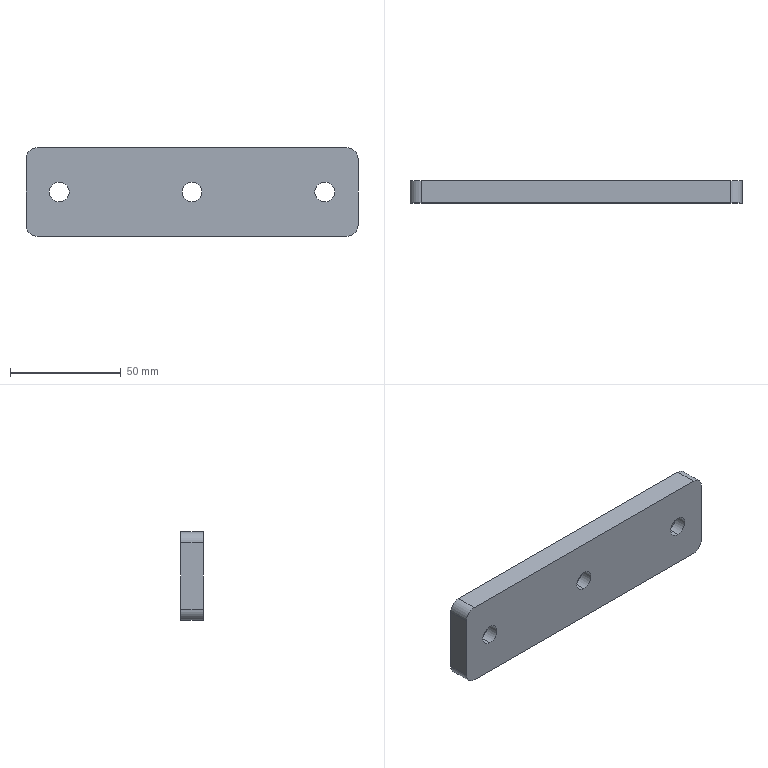Part | SolidWorks | features LPattern 2, Extrusion 1, Fillet 1, HoleWzd 1, ICE 1 | 1 solid | 22 faces | box 150 x 10 x 40 mm | volume 56843 mm3 | cylinder 10 | cone 6 | plane 6 | commonest cylinder face diameters 9 x6 10 x4
STEP:
#1=CARTESIAN_POINT('',(75.,5.7,-24.5));
#2=VERTEX_POINT('',#1);
#3=CARTESIAN_POINT('',(75.,5.7,-15.5));
#4=VERTEX_POINT('',#3);
#5=CARTESIAN_POINT('',(75.,5.7,-20.));
#6=DIRECTION('',(0.,1.,0.));
#7=DIRECTION('',(0.,0.,1.));
#8=AXIS2_PLACEMENT_3D('',#5,#6,#7);
#9=CIRCLE('',#8,4.5);
#10=EDGE_CURVE('',#2,#4,#9,.T.);
#11=ORIENTED_EDGE('',*,*,#10,.F.);
#12=CARTESIAN_POINT('',(75.,10.,-28.8));
#13=VERTEX_POINT('',#12);
#14=CARTESIAN_POINT('',(75.,10.,-28.8));
#15=DIRECTION('',(0.,0.7071,-0.7071));
#16=VECTOR('',#15,1000.);
#17=LINE('',#14,#16);
#18=EDGE_CURVE('',#2,#13,#17,.T.);
#19=ORIENTED_EDGE('',*,*,#18,.T.);
#20=CARTESIAN_POINT('',(75.,10.,-11.2));
#21=VERTEX_POINT('',#20);
#22=CARTESIAN_POINT('',(75.,10.,-20.));
#23=DIRECTION('',(0.,1.,0.));
#24=DIRECTION('',(0.,0.,1.));
#25=AXIS2_PLACEMENT_3D('',#22,#23,#24);
#26=CIRCLE('',#25,8.8);
#27=EDGE_CURVE('',#13,#21,#26,.T.);
#28=ORIENTED_EDGE('',*,*,#27,.T.);
#29=CARTESIAN_POINT('',(75.,10.,-11.2));
#30=DIRECTION('',(0.,0.7071,0.7071));
#31=VECTOR('',#30,1000.);
#32=LINE('',#29,#31);
#33=EDGE_CURVE('',#4,#21,#32,.T.);
#34=ORIENTED_EDGE('',*,*,#33,.F.);
#35=EDGE_LOOP('',(#11,#19,#28,#34));
#36=FACE_OUTER_BOUND('',#35,.T.);
#37=CARTESIAN_POINT('',(75.,10.,-20.));
#38=DIRECTION('',(0.,1.,0.));
#39=DIRECTION('',(0.,0.,1.));
#40=AXIS2_PLACEMENT_3D('',#37,#38,#39);
#41=CONICAL_SURFACE('',#40,8.8,0.7854);
#42=ADVANCED_FACE('',(#36),#41,.F.);
#43=CARTESIAN_POINT('',(75.,0.,-15.5));
#44=VERTEX_POINT('',#43);
#45=CARTESIAN_POINT('',(75.,0.,-24.5));
#46=VERTEX_POINT('',#45);
#47=CARTESIAN_POINT('',(75.,0.,-20.));
#48=DIRECTION('',(0.,-1.,0.));
#49=DIRECTION('',(0.,0.,-1.));
#50=AXIS2_PLACEMENT_3D('',#47,#48,#49);
#51=CIRCLE('',#50,4.5);
#52=EDGE_CURVE('',#44,#46,#51,.T.);
#53=ORIENTED_EDGE('',*,*,#52,.T.);
#54=CARTESIAN_POINT('',(75.,10.,-24.5));
#55=DIRECTION('',(0.,1.,0.));
#56=VECTOR('',#55,1000.);
#57=LINE('',#54,#56);
#58=EDGE_CURVE('',#46,#2,#57,.T.);
#59=ORIENTED_EDGE('',*,*,#58,.T.);
#60=ORIENTED_EDGE('',*,*,#10,.T.);
#61=CARTESIAN_POINT('',(75.,10.,-15.5));
#62=DIRECTION('',(0.,1.,0.));
#63=VECTOR('',#62,1000.);
#64=LINE('',#61,#63);
#65=EDGE_CURVE('',#44,#4,#64,.T.);
#66=ORIENTED_EDGE('',*,*,#65,.F.);
#67=EDGE_LOOP('',(#53,#59,#60,#66));
#68=FACE_OUTER_BOUND('',#67,.T.);
#69=CARTESIAN_POINT('',(75.,10.,-20.));
#70=DIRECTION('',(0.,1.,0.));
#71=DIRECTION('',(0.,0.,1.));
#72=AXIS2_PLACEMENT_3D('',#69,#70,#71);
#73=CYLINDRICAL_SURFACE('',#72,4.5);
#74=ADVANCED_FACE('',(#68),#73,.F.);
#75=CARTESIAN_POINT('',(15.,5.7,-24.5));
#76=VERTEX_POINT('',#75);
#77=CARTESIAN_POINT('',(15.,5.7,-15.5));
#78=VERTEX_POINT('',#77);
#79=CARTESIAN_POINT('',(15.,5.7,-20.));
#80=DIRECTION('',(0.,1.,0.));
#81=DIRECTION('',(0.,0.,1.));
#82=AXIS2_PLACEMENT_3D('',#79,#80,#81);
#83=CIRCLE('',#82,4.5);
#84=EDGE_CURVE('',#76,#78,#83,.T.);
#85=ORIENTED_EDGE('',*,*,#84,.F.);
#86=CARTESIAN_POINT('',(15.,10.,-28.8));
#87=VERTEX_POINT('',#86);
#88=CARTESIAN_POINT('',(15.,10.,-28.8));
#89=DIRECTION('',(0.,0.7071,-0.7071));
#90=VECTOR('',#89,1000.);
#91=LINE('',#88,#90);
#92=EDGE_CURVE('',#76,#87,#91,.T.);
#93=ORIENTED_EDGE('',*,*,#92,.T.);
#94=CARTESIAN_POINT('',(15.,10.,-11.2));
#95=VERTEX_POINT('',#94);
#96=CARTESIAN_POINT('',(15.,10.,-20.));
#97=DIRECTION('',(0.,1.,0.));
#98=DIRECTION('',(0.,0.,1.));
#99=AXIS2_PLACEMENT_3D('',#96,#97,#98);
#100=CIRCLE('',#99,8.8);
#101=EDGE_CURVE('',#87,#95,#100,.T.);
#102=ORIENTED_EDGE('',*,*,#101,.T.);
#103=CARTESIAN_POINT('',(15.,10.,-11.2));
#104=DIRECTION('',(0.,0.7071,0.7071));
#105=VECTOR('',#104,1000.);
#106=LINE('',#103,#105);
#107=EDGE_CURVE('',#78,#95,#106,.T.);
#108=ORIENTED_EDGE('',*,*,#107,.F.);
#109=EDGE_LOOP('',(#85,#93,#102,#108));
#110=FACE_OUTER_BOUND('',#109,.T.);
#111=CARTESIAN_POINT('',(15.,10.,-20.));
#112=DIRECTION('',(0.,1.,0.));
#113=DIRECTION('',(0.,0.,1.));
#114=AXIS2_PLACEMENT_3D('',#111,#112,#113);
#115=CONICAL_SURFACE('',#114,8.8,0.7854);
#116=ADVANCED_FACE('',(#110),#115,.F.);
#117=CARTESIAN_POINT('',(15.,0.,-15.5));
#118=VERTEX_POINT('',#117);
#119=CARTESIAN_POINT('',(15.,0.,-24.5));
#120=VERTEX_POINT('',#119);
#121=CARTESIAN_POINT('',(15.,0.,-20.));
#122=DIRECTION('',(0.,-1.,0.));
#123=DIRECTION('',(0.,0.,-1.));
#124=AXIS2_PLACEMENT_3D('',#121,#122,#123);
#125=CIRCLE('',#124,4.5);
#126=EDGE_CURVE('',#118,#120,#125,.T.);
#127=ORIENTED_EDGE('',*,*,#126,.T.);
#128=CARTESIAN_POINT('',(15.,10.,-24.5));
#129=DIRECTION('',(0.,1.,0.));
#130=VECTOR('',#129,1000.);
#131=LINE('',#128,#130);
#132=EDGE_CURVE('',#120,#76,#131,.T.);
#133=ORIENTED_EDGE('',*,*,#132,.T.);
#134=ORIENTED_EDGE('',*,*,#84,.T.);
#135=CARTESIAN_POINT('',(15.,10.,-15.5));
#136=DIRECTION('',(0.,1.,0.));
#137=VECTOR('',#136,1000.);
#138=LINE('',#135,#137);
#139=EDGE_CURVE('',#118,#78,#138,.T.);
#140=ORIENTED_EDGE('',*,*,#139,.F.);
#141=EDGE_LOOP('',(#127,#133,#134,#140));
#142=FACE_OUTER_BOUND('',#141,.T.);
#143=CARTESIAN_POINT('',(15.,10.,-20.));
#144=DIRECTION('',(0.,1.,0.));
#145=DIRECTION('',(0.,0.,1.));
#146=AXIS2_PLACEMENT_3D('',#143,#144,#145);
#147=CYLINDRICAL_SURFACE('',#146,4.5);
#148=ADVANCED_FACE('',(#142),#147,.F.);
#149=CARTESIAN_POINT('',(135.,5.7,-24.5));
#150=VERTEX_POINT('',#149);
#151=CARTESIAN_POINT('',(135.,5.7,-15.5));
#152=VERTEX_POINT('',#151);
#153=CARTESIAN_POINT('',(135.,5.7,-20.));
#154=DIRECTION('',(0.,1.,0.));
#155=DIRECTION('',(0.,0.,1.));
#156=AXIS2_PLACEMENT_3D('',#153,#154,#155);
#157=CIRCLE('',#156,4.5);
#158=EDGE_CURVE('',#150,#152,#157,.T.);
#159=ORIENTED_EDGE('',*,*,#158,.F.);
#160=CARTESIAN_POINT('',(135.,10.,-28.8));
#161=VERTEX_POINT('',#160);
#162=CARTESIAN_POINT('',(135.,10.,-28.8));
#163=DIRECTION('',(0.,0.7071,-0.7071));
#164=VECTOR('',#163,1000.);
#165=LINE('',#162,#164);
#166=EDGE_CURVE('',#150,#161,#165,.T.);
#167=ORIENTED_EDGE('',*,*,#166,.T.);
#168=CARTESIAN_POINT('',(135.,10.,-11.2));
#169=VERTEX_POINT('',#168);
#170=CARTESIAN_POINT('',(135.,10.,-20.));
#171=DIRECTION('',(0.,1.,0.));
#172=DIRECTION('',(0.,0.,1.));
#173=AXIS2_PLACEMENT_3D('',#170,#171,#172);
#174=CIRCLE('',#173,8.8);
#175=EDGE_CURVE('',#161,#169,#174,.T.);
#176=ORIENTED_EDGE('',*,*,#175,.T.);
#177=CARTESIAN_POINT('',(135.,10.,-11.2));
#178=DIRECTION('',(0.,0.7071,0.7071));
#179=VECTOR('',#178,1000.);
#180=LINE('',#177,#179);
#181=EDGE_CURVE('',#152,#169,#180,.T.);
#182=ORIENTED_EDGE('',*,*,#181,.F.);
#183=EDGE_LOOP('',(#159,#167,#176,#182));
#184=FACE_OUTER_BOUND('',#183,.T.);
#185=CARTESIAN_POINT('',(135.,10.,-20.));
#186=DIRECTION('',(0.,1.,0.));
#187=DIRECTION('',(0.,0.,1.));
#188=AXIS2_PLACEMENT_3D('',#185,#186,#187);
#189=CONICAL_SURFACE('',#188,8.8,0.7854);
#190=ADVANCED_FACE('',(#184),#189,.F.);
#191=CARTESIAN_POINT('',(135.,0.,-15.5));
#192=VERTEX_POINT('',#191);
#193=CARTESIAN_POINT('',(135.,0.,-24.5));
#194=VERTEX_POINT('',#193);
#195=CARTESIAN_POINT('',(135.,0.,-20.));
#196=DIRECTION('',(0.,-1.,0.));
#197=DIRECTION('',(0.,0.,-1.));
#198=AXIS2_PLACEMENT_3D('',#195,#196,#197);
#199=CIRCLE('',#198,4.5);
#200=EDGE_CURVE('',#192,#194,#199,.T.);
#201=ORIENTED_EDGE('',*,*,#200,.T.);
#202=CARTESIAN_POINT('',(135.,10.,-24.5));
#203=DIRECTION('',(0.,1.,0.));
#204=VECTOR('',#203,1000.);
#205=LINE('',#202,#204);
#206=EDGE_CURVE('',#194,#150,#205,.T.);
#207=ORIENTED_EDGE('',*,*,#206,.T.);
#208=ORIENTED_EDGE('',*,*,#158,.T.);
#209=CARTESIAN_POINT('',(135.,10.,-15.5));
#210=DIRECTION('',(0.,1.,0.));
#211=VECTOR('',#210,1000.);
#212=LINE('',#209,#211);
#213=EDGE_CURVE('',#192,#152,#212,.T.);
#214=ORIENTED_EDGE('',*,*,#213,.F.);
#215=EDGE_LOOP('',(#201,#207,#208,#214));
#216=FACE_OUTER_BOUND('',#215,.T.);
#217=CARTESIAN_POINT('',(135.,10.,-20.));
#218=DIRECTION('',(0.,1.,0.));
#219=DIRECTION('',(0.,0.,1.));
#220=AXIS2_PLACEMENT_3D('',#217,#218,#219);
#221=CYLINDRICAL_SURFACE('',#220,4.5);
#222=ADVANCED_FACE('',(#216),#221,.F.);
#223=CARTESIAN_POINT('',(0.,10.,-35.));
#224=VERTEX_POINT('',#223);
#225=CARTESIAN_POINT('',(0.,10.,-5.));
#226=VERTEX_POINT('',#225);
#227=CARTESIAN_POINT('',(0.,10.,0.));
#228=DIRECTION('',(0.,0.,1.));
#229=VECTOR('',#228,1000.);
#230=LINE('',#227,#229);
#231=EDGE_CURVE('',#224,#226,#230,.T.);
#232=ORIENTED_EDGE('',*,*,#231,.F.);
#233=CARTESIAN_POINT('',(0.,0.,-35.));
#234=VERTEX_POINT('',#233);
#235=CARTESIAN_POINT('',(0.,10.,-35.));
#236=DIRECTION('',(0.,-1.,0.));
#237=VECTOR('',#236,1000.);
#238=LINE('',#235,#237);
#239=EDGE_CURVE('',#224,#234,#238,.T.);
#240=ORIENTED_EDGE('',*,*,#239,.T.);
#241=CARTESIAN_POINT('',(0.,0.,-5.));
#242=VERTEX_POINT('',#241);
#243=CARTESIAN_POINT('',(0.,0.,0.));
#244=DIRECTION('',(0.,0.,1.));
#245=VECTOR('',#244,1000.);
#246=LINE('',#243,#245);
#247=EDGE_CURVE('',#234,#242,#246,.T.);
#248=ORIENTED_EDGE('',*,*,#247,.T.);
#249=CARTESIAN_POINT('',(0.,10.,-5.));
#250=DIRECTION('',(0.,1.,0.));
#251=VECTOR('',#250,1000.);
#252=LINE('',#249,#251);
#253=EDGE_CURVE('',#242,#226,#252,.T.);
#254=ORIENTED_EDGE('',*,*,#253,.T.);
#255=EDGE_LOOP('',(#232,#240,#248,#254));
#256=FACE_OUTER_BOUND('',#255,.T.);
#257=CARTESIAN_POINT('',(0.,10.,0.));
#258=DIRECTION('',(1.,0.,0.));
#259=DIRECTION('',(0.,0.,-1.));
#260=AXIS2_PLACEMENT_3D('',#257,#258,#259);
#261=PLANE('',#260);
#262=ADVANCED_FACE('',(#256),#261,.F.);
#263=CARTESIAN_POINT('',(5.,0.,0.));
#264=VERTEX_POINT('',#263);
#265=CARTESIAN_POINT('',(145.,0.,0.));
#266=VERTEX_POINT('',#265);
#267=CARTESIAN_POINT('',(0.,0.,0.));
#268=DIRECTION('',(1.,0.,0.));
#269=VECTOR('',#268,1000.);
#270=LINE('',#267,#269);
#271=EDGE_CURVE('',#264,#266,#270,.T.);
#272=ORIENTED_EDGE('',*,*,#271,.T.);
#273=CARTESIAN_POINT('',(145.,10.,0.));
#274=VERTEX_POINT('',#273);
#275=CARTESIAN_POINT('',(145.,10.,0.));
#276=DIRECTION('',(0.,1.,0.));
#277=VECTOR('',#276,1000.);
#278=LINE('',#275,#277);
#279=EDGE_CURVE('',#266,#274,#278,.T.);
#280=ORIENTED_EDGE('',*,*,#279,.T.);
#281=CARTESIAN_POINT('',(5.,10.,0.));
#282=VERTEX_POINT('',#281);
#283=CARTESIAN_POINT('',(0.,10.,0.));
#284=DIRECTION('',(1.,0.,0.));
#285=VECTOR('',#284,1000.);
#286=LINE('',#283,#285);
#287=EDGE_CURVE('',#282,#274,#286,.T.);
#288=ORIENTED_EDGE('',*,*,#287,.F.);
#289=CARTESIAN_POINT('',(5.,10.,0.));
#290=DIRECTION('',(0.,-1.,0.));
#291=VECTOR('',#290,1000.);
#292=LINE('',#289,#291);
#293=EDGE_CURVE('',#282,#264,#292,.T.);
#294=ORIENTED_EDGE('',*,*,#293,.T.);
#295=EDGE_LOOP('',(#272,#280,#288,#294));
#296=FACE_OUTER_BOUND('',#295,.T.);
#297=CARTESIAN_POINT('',(0.,10.,0.));
#298=DIRECTION('',(0.,0.,-1.));
#299=DIRECTION('',(-1.,0.,0.));
#300=AXIS2_PLACEMENT_3D('',#297,#298,#299);
#301=PLANE('',#300);
#302=ADVANCED_FACE('',(#296),#301,.F.);
#303=CARTESIAN_POINT('',(150.,0.,-5.));
#304=VERTEX_POINT('',#303);
#305=CARTESIAN_POINT('',(150.,0.,-35.));
#306=VERTEX_POINT('',#305);
#307=CARTESIAN_POINT('',(150.,0.,0.));
#308=DIRECTION('',(0.,0.,-1.));
#309=VECTOR('',#308,1000.);
#310=LINE('',#307,#309);
#311=EDGE_CURVE('',#304,#306,#310,.T.);
#312=ORIENTED_EDGE('',*,*,#311,.T.);
#313=CARTESIAN_POINT('',(150.,10.,-35.));
#314=VERTEX_POINT('',#313);
#315=CARTESIAN_POINT('',(150.,10.,-35.));
#316=DIRECTION('',(0.,1.,0.));
#317=VECTOR('',#316,1000.);
#318=LINE('',#315,#317);
#319=EDGE_CURVE('',#306,#314,#318,.T.);
#320=ORIENTED_EDGE('',*,*,#319,.T.);
#321=CARTESIAN_POINT('',(150.,10.,-5.));
#322=VERTEX_POINT('',#321);
#323=CARTESIAN_POINT('',(150.,10.,0.));
#324=DIRECTION('',(0.,0.,-1.));
#325=VECTOR('',#324,1000.);
#326=LINE('',#323,#325);
#327=EDGE_CURVE('',#322,#314,#326,.T.);
#328=ORIENTED_EDGE('',*,*,#327,.F.);
#329=CARTESIAN_POINT('',(150.,10.,-5.));
#330=DIRECTION('',(0.,-1.,0.));
#331=VECTOR('',#330,1000.);
#332=LINE('',#329,#331);
#333=EDGE_CURVE('',#322,#304,#332,.T.);
#334=ORIENTED_EDGE('',*,*,#333,.T.);
#335=EDGE_LOOP('',(#312,#320,#328,#334));
#336=FACE_OUTER_BOUND('',#335,.T.);
#337=CARTESIAN_POINT('',(150.,10.,0.));
#338=DIRECTION('',(-1.,0.,0.));
#339=DIRECTION('',(0.,0.,1.));
#340=AXIS2_PLACEMENT_3D('',#337,#338,#339);
#341=PLANE('',#340);
#342=ADVANCED_FACE('',(#336),#341,.F.);
#343=CARTESIAN_POINT('',(145.,0.,-40.));
#344=VERTEX_POINT('',#343);
#345=CARTESIAN_POINT('',(5.,0.,-40.));
#346=VERTEX_POINT('',#345);
#347=CARTESIAN_POINT('',(0.,0.,-40.));
#348=DIRECTION('',(-1.,0.,0.));
#349=VECTOR('',#348,1000.);
#350=LINE('',#347,#349);
#351=EDGE_CURVE('',#344,#346,#350,.T.);
#352=ORIENTED_EDGE('',*,*,#351,.T.);
#353=CARTESIAN_POINT('',(5.,10.,-40.));
#354=VERTEX_POINT('',#353);
#355=CARTESIAN_POINT('',(5.,10.,-40.));
#356=DIRECTION('',(0.,1.,0.));
#357=VECTOR('',#356,1000.);
#358=LINE('',#355,#357);
#359=EDGE_CURVE('',#346,#354,#358,.T.);
#360=ORIENTED_EDGE('',*,*,#359,.T.);
#361=CARTESIAN_POINT('',(145.,10.,-40.));
#362=VERTEX_POINT('',#361);
#363=CARTESIAN_POINT('',(0.,10.,-40.));
#364=DIRECTION('',(-1.,0.,0.));
#365=VECTOR('',#364,1000.);
#366=LINE('',#363,#365);
#367=EDGE_CURVE('',#362,#354,#366,.T.);
#368=ORIENTED_EDGE('',*,*,#367,.F.);
#369=CARTESIAN_POINT('',(145.,10.,-40.));
#370=DIRECTION('',(0.,-1.,0.));
#371=VECTOR('',#370,1000.);
#372=LINE('',#369,#371);
#373=EDGE_CURVE('',#362,#344,#372,.T.);
#374=ORIENTED_EDGE('',*,*,#373,.T.);
#375=EDGE_LOOP('',(#352,#360,#368,#374));
#376=FACE_OUTER_BOUND('',#375,.T.);
#377=CARTESIAN_POINT('',(0.,10.,-40.));
#378=DIRECTION('',(0.,0.,1.));
#379=DIRECTION('',(1.,0.,0.));
#380=AXIS2_PLACEMENT_3D('',#377,#378,#379);
#381=PLANE('',#380);
#382=ADVANCED_FACE('',(#376),#381,.F.);
#383=CARTESIAN_POINT('',(75.,10.,-20.));
#384=DIRECTION('',(0.,1.,0.));
#385=DIRECTION('',(0.,0.,1.));
#386=AXIS2_PLACEMENT_3D('',#383,#384,#385);
#387=CIRCLE('',#386,8.8);
#388=EDGE_CURVE('',#21,#13,#387,.T.);
#389=ORIENTED_EDGE('',*,*,#388,.F.);
#390=ORIENTED_EDGE('',*,*,#27,.F.);
#391=EDGE_LOOP('',(#389,#390));
#392=FACE_BOUND('',#391,.T.);
#393=CARTESIAN_POINT('',(15.,10.,-20.));
#394=DIRECTION('',(0.,1.,0.));
#395=DIRECTION('',(0.,0.,1.));
#396=AXIS2_PLACEMENT_3D('',#393,#394,#395);
#397=CIRCLE('',#396,8.8);
#398=EDGE_CURVE('',#95,#87,#397,.T.);
#399=ORIENTED_EDGE('',*,*,#398,.F.);
#400=ORIENTED_EDGE('',*,*,#101,.F.);
#401=EDGE_LOOP('',(#399,#400));
#402=FACE_BOUND('',#401,.T.);
#403=CARTESIAN_POINT('',(135.,10.,-20.));
#404=DIRECTION('',(0.,1.,0.));
#405=DIRECTION('',(0.,0.,1.));
#406=AXIS2_PLACEMENT_3D('',#403,#404,#405);
#407=CIRCLE('',#406,8.8);
#408=EDGE_CURVE('',#169,#161,#407,.T.);
#409=ORIENTED_EDGE('',*,*,#408,.F.);
#410=ORIENTED_EDGE('',*,*,#175,.F.);
#411=EDGE_LOOP('',(#409,#410));
#412=FACE_BOUND('',#411,.T.);
#413=ORIENTED_EDGE('',*,*,#367,.T.);
#414=CARTESIAN_POINT('',(5.,10.,-35.));
#415=DIRECTION('',(0.,1.,0.));
#416=DIRECTION('',(0.,0.,-1.));
#417=AXIS2_PLACEMENT_3D('',#414,#415,#416);
#418=CIRCLE('',#417,5.);
#419=EDGE_CURVE('',#354,#224,#418,.T.);
#420=ORIENTED_EDGE('',*,*,#419,.T.);
#421=ORIENTED_EDGE('',*,*,#231,.T.);
#422=CARTESIAN_POINT('',(5.,10.,-5.));
#423=DIRECTION('',(0.,1.,0.));
#424=DIRECTION('',(0.,0.,-1.));
#425=AXIS2_PLACEMENT_3D('',#422,#423,#424);
#426=CIRCLE('',#425,5.);
#427=EDGE_CURVE('',#226,#282,#426,.T.);
#428=ORIENTED_EDGE('',*,*,#427,.T.);
#429=ORIENTED_EDGE('',*,*,#287,.T.);
#430=CARTESIAN_POINT('',(145.,10.,-5.));
#431=DIRECTION('',(0.,1.,0.));
#432=DIRECTION('',(0.,0.,-1.));
#433=AXIS2_PLACEMENT_3D('',#430,#431,#432);
#434=CIRCLE('',#433,5.);
#435=EDGE_CURVE('',#274,#322,#434,.T.);
#436=ORIENTED_EDGE('',*,*,#435,.T.);
#437=ORIENTED_EDGE('',*,*,#327,.T.);
#438=CARTESIAN_POINT('',(145.,10.,-35.));
#439=DIRECTION('',(0.,1.,0.));
#440=DIRECTION('',(0.,0.,-1.));
#441=AXIS2_PLACEMENT_3D('',#438,#439,#440);
#442=CIRCLE('',#441,5.);
#443=EDGE_CURVE('',#314,#362,#442,.T.);
#444=ORIENTED_EDGE('',*,*,#443,.T.);
#445=EDGE_LOOP('',(#413,#420,#421,#428,#429,#436,#437,#444));
#446=FACE_OUTER_BOUND('',#445,.T.);
#447=CARTESIAN_POINT('',(0.,10.,0.));
#448=DIRECTION('',(0.,-1.,0.));
#449=DIRECTION('',(0.,0.,-1.));
#450=AXIS2_PLACEMENT_3D('',#447,#448,#449);
#451=PLANE('',#450);
#452=ADVANCED_FACE('',(#392,#402,#412,#446),#451,.F.);
#453=ORIENTED_EDGE('',*,*,#52,.F.);
#454=CARTESIAN_POINT('',(75.,0.,-20.));
#455=DIRECTION('',(0.,-1.,0.));
#456=DIRECTION('',(0.,0.,-1.));
#457=AXIS2_PLACEMENT_3D('',#454,#455,#456);
#458=CIRCLE('',#457,4.5);
#459=EDGE_CURVE('',#46,#44,#458,.T.);
#460=ORIENTED_EDGE('',*,*,#459,.F.);
#461=EDGE_LOOP('',(#453,#460));
#462=FACE_BOUND('',#461,.T.);
#463=ORIENTED_EDGE('',*,*,#126,.F.);
#464=CARTESIAN_POINT('',(15.,0.,-20.));
#465=DIRECTION('',(0.,-1.,0.));
#466=DIRECTION('',(0.,0.,-1.));
#467=AXIS2_PLACEMENT_3D('',#464,#465,#466);
#468=CIRCLE('',#467,4.5);
#469=EDGE_CURVE('',#120,#118,#468,.T.);
#470=ORIENTED_EDGE('',*,*,#469,.F.);
#471=EDGE_LOOP('',(#463,#470));
#472=FACE_BOUND('',#471,.T.);
#473=ORIENTED_EDGE('',*,*,#200,.F.);
#474=CARTESIAN_POINT('',(135.,0.,-20.));
#475=DIRECTION('',(0.,-1.,0.));
#476=DIRECTION('',(0.,0.,-1.));
#477=AXIS2_PLACEMENT_3D('',#474,#475,#476);
#478=CIRCLE('',#477,4.5);
#479=EDGE_CURVE('',#194,#192,#478,.T.);
#480=ORIENTED_EDGE('',*,*,#479,.F.);
#481=EDGE_LOOP('',(#473,#480));
#482=FACE_BOUND('',#481,.T.);
#483=ORIENTED_EDGE('',*,*,#247,.F.);
#484=CARTESIAN_POINT('',(5.,0.,-35.));
#485=DIRECTION('',(0.,-1.,0.));
#486=DIRECTION('',(0.,0.,-1.));
#487=AXIS2_PLACEMENT_3D('',#484,#485,#486);
#488=CIRCLE('',#487,5.);
#489=EDGE_CURVE('',#234,#346,#488,.T.);
#490=ORIENTED_EDGE('',*,*,#489,.T.);
#491=ORIENTED_EDGE('',*,*,#351,.F.);
#492=CARTESIAN_POINT('',(145.,0.,-35.));
#493=DIRECTION('',(0.,-1.,0.));
#494=DIRECTION('',(0.,0.,-1.));
#495=AXIS2_PLACEMENT_3D('',#492,#493,#494);
#496=CIRCLE('',#495,5.);
#497=EDGE_CURVE('',#344,#306,#496,.T.);
#498=ORIENTED_EDGE('',*,*,#497,.T.);
#499=ORIENTED_EDGE('',*,*,#311,.F.);
#500=CARTESIAN_POINT('',(145.,0.,-5.));
#501=DIRECTION('',(0.,-1.,0.));
#502=DIRECTION('',(0.,0.,-1.));
#503=AXIS2_PLACEMENT_3D('',#500,#501,#502);
#504=CIRCLE('',#503,5.);
#505=EDGE_CURVE('',#304,#266,#504,.T.);
#506=ORIENTED_EDGE('',*,*,#505,.T.);
#507=ORIENTED_EDGE('',*,*,#271,.F.);
#508=CARTESIAN_POINT('',(5.,0.,-5.));
#509=DIRECTION('',(0.,-1.,0.));
#510=DIRECTION('',(0.,0.,-1.));
#511=AXIS2_PLACEMENT_3D('',#508,#509,#510);
#512=CIRCLE('',#511,5.);
#513=EDGE_CURVE('',#264,#242,#512,.T.);
#514=ORIENTED_EDGE('',*,*,#513,.T.);
#515=EDGE_LOOP('',(#483,#490,#491,#498,#499,#506,#507,#514));
#516=FACE_OUTER_BOUND('',#515,.T.);
#517=CARTESIAN_POINT('',(0.,0.,0.));
#518=DIRECTION('',(0.,-1.,0.));
#519=DIRECTION('',(0.,0.,-1.));
#520=AXIS2_PLACEMENT_3D('',#517,#518,#519);
#521=PLANE('',#520);
#522=ADVANCED_FACE('',(#462,#472,#482,#516),#521,.T.);
#523=ORIENTED_EDGE('',*,*,#419,.F.);
#524=ORIENTED_EDGE('',*,*,#359,.F.);
#525=ORIENTED_EDGE('',*,*,#489,.F.);
#526=ORIENTED_EDGE('',*,*,#239,.F.);
#527=EDGE_LOOP('',(#523,#524,#525,#526));
#528=FACE_OUTER_BOUND('',#527,.T.);
#529=CARTESIAN_POINT('',(5.,10.,-35.));
#530=DIRECTION('',(0.,-1.,0.));
#531=DIRECTION('',(0.,0.,-1.));
#532=AXIS2_PLACEMENT_3D('',#529,#530,#531);
#533=CYLINDRICAL_SURFACE('',#532,5.);
#534=ADVANCED_FACE('',(#528),#533,.T.);
#535=ORIENTED_EDGE('',*,*,#443,.F.);
#536=ORIENTED_EDGE('',*,*,#319,.F.);
#537=ORIENTED_EDGE('',*,*,#497,.F.);
#538=ORIENTED_EDGE('',*,*,#373,.F.);
#539=EDGE_LOOP('',(#535,#536,#537,#538));
#540=FACE_OUTER_BOUND('',#539,.T.);
#541=CARTESIAN_POINT('',(145.,10.,-35.));
#542=DIRECTION('',(0.,-1.,0.));
#543=DIRECTION('',(0.,0.,-1.));
#544=AXIS2_PLACEMENT_3D('',#541,#542,#543);
#545=CYLINDRICAL_SURFACE('',#544,5.);
#546=ADVANCED_FACE('',(#540),#545,.T.);
#547=ORIENTED_EDGE('',*,*,#435,.F.);
#548=ORIENTED_EDGE('',*,*,#279,.F.);
#549=ORIENTED_EDGE('',*,*,#505,.F.);
#550=ORIENTED_EDGE('',*,*,#333,.F.);
#551=EDGE_LOOP('',(#547,#548,#549,#550));
#552=FACE_OUTER_BOUND('',#551,.T.);
#553=CARTESIAN_POINT('',(145.,10.,-5.));
#554=DIRECTION('',(0.,-1.,0.));
#555=DIRECTION('',(0.,0.,-1.));
#556=AXIS2_PLACEMENT_3D('',#553,#554,#555);
#557=CYLINDRICAL_SURFACE('',#556,5.);
#558=ADVANCED_FACE('',(#552),#557,.T.);
#559=ORIENTED_EDGE('',*,*,#427,.F.);
#560=ORIENTED_EDGE('',*,*,#253,.F.);
#561=ORIENTED_EDGE('',*,*,#513,.F.);
#562=ORIENTED_EDGE('',*,*,#293,.F.);
#563=EDGE_LOOP('',(#559,#560,#561,#562));
#564=FACE_OUTER_BOUND('',#563,.T.);
#565=CARTESIAN_POINT('',(5.,10.,-5.));
#566=DIRECTION('',(0.,-1.,0.));
#567=DIRECTION('',(0.,0.,-1.));
#568=AXIS2_PLACEMENT_3D('',#565,#566,#567);
#569=CYLINDRICAL_SURFACE('',#568,5.);
#570=ADVANCED_FACE('',(#564),#569,.T.);
#571=ORIENTED_EDGE('',*,*,#206,.F.);
#572=ORIENTED_EDGE('',*,*,#479,.T.);
#573=ORIENTED_EDGE('',*,*,#213,.T.);
#574=CARTESIAN_POINT('',(135.,5.7,-20.));
#575=DIRECTION('',(0.,1.,0.));
#576=DIRECTION('',(0.,0.,1.));
#577=AXIS2_PLACEMENT_3D('',#574,#575,#576);
#578=CIRCLE('',#577,4.5);
#579=EDGE_CURVE('',#152,#150,#578,.T.);
#580=ORIENTED_EDGE('',*,*,#579,.T.);
#581=EDGE_LOOP('',(#571,#572,#573,#580));
#582=FACE_OUTER_BOUND('',#581,.T.);
#583=CARTESIAN_POINT('',(135.,10.,-20.));
#584=DIRECTION('',(0.,1.,0.));
#585=DIRECTION('',(0.,0.,1.));
#586=AXIS2_PLACEMENT_3D('',#583,#584,#585);
#587=CYLINDRICAL_SURFACE('',#586,4.5);
#588=ADVANCED_FACE('',(#582),#587,.F.);
#589=ORIENTED_EDGE('',*,*,#166,.F.);
#590=ORIENTED_EDGE('',*,*,#579,.F.);
#591=ORIENTED_EDGE('',*,*,#181,.T.);
#592=ORIENTED_EDGE('',*,*,#408,.T.);
#593=EDGE_LOOP('',(#589,#590,#591,#592));
#594=FACE_OUTER_BOUND('',#593,.T.);
#595=CARTESIAN_POINT('',(135.,10.,-20.));
#596=DIRECTION('',(0.,1.,0.));
#597=DIRECTION('',(0.,0.,1.));
#598=AXIS2_PLACEMENT_3D('',#595,#596,#597);
#599=CONICAL_SURFACE('',#598,8.8,0.7854);
#600=ADVANCED_FACE('',(#594),#599,.F.);
#601=ORIENTED_EDGE('',*,*,#132,.F.);
#602=ORIENTED_EDGE('',*,*,#469,.T.);
#603=ORIENTED_EDGE('',*,*,#139,.T.);
#604=CARTESIAN_POINT('',(15.,5.7,-20.));
#605=DIRECTION('',(0.,1.,0.));
#606=DIRECTION('',(0.,0.,1.));
#607=AXIS2_PLACEMENT_3D('',#604,#605,#606);
#608=CIRCLE('',#607,4.5);
#609=EDGE_CURVE('',#78,#76,#608,.T.);
#610=ORIENTED_EDGE('',*,*,#609,.T.);
#611=EDGE_LOOP('',(#601,#602,#603,#610));
#612=FACE_OUTER_BOUND('',#611,.T.);
#613=CARTESIAN_POINT('',(15.,10.,-20.));
#614=DIRECTION('',(0.,1.,0.));
#615=DIRECTION('',(0.,0.,1.));
#616=AXIS2_PLACEMENT_3D('',#613,#614,#615);
#617=CYLINDRICAL_SURFACE('',#616,4.5);
#618=ADVANCED_FACE('',(#612),#617,.F.);
#619=ORIENTED_EDGE('',*,*,#92,.F.);
#620=ORIENTED_EDGE('',*,*,#609,.F.);
#621=ORIENTED_EDGE('',*,*,#107,.T.);
#622=ORIENTED_EDGE('',*,*,#398,.T.);
#623=EDGE_LOOP('',(#619,#620,#621,#622));
#624=FACE_OUTER_BOUND('',#623,.T.);
#625=CARTESIAN_POINT('',(15.,10.,-20.));
#626=DIRECTION('',(0.,1.,0.));
#627=DIRECTION('',(0.,0.,1.));
#628=AXIS2_PLACEMENT_3D('',#625,#626,#627);
#629=CONICAL_SURFACE('',#628,8.8,0.7854);
#630=ADVANCED_FACE('',(#624),#629,.F.);
#631=ORIENTED_EDGE('',*,*,#58,.F.);
#632=ORIENTED_EDGE('',*,*,#459,.T.);
#633=ORIENTED_EDGE('',*,*,#65,.T.);
#634=CARTESIAN_POINT('',(75.,5.7,-20.));
#635=DIRECTION('',(0.,1.,0.));
#636=DIRECTION('',(0.,0.,1.));
#637=AXIS2_PLACEMENT_3D('',#634,#635,#636);
#638=CIRCLE('',#637,4.5);
#639=EDGE_CURVE('',#4,#2,#638,.T.);
#640=ORIENTED_EDGE('',*,*,#639,.T.);
#641=EDGE_LOOP('',(#631,#632,#633,#640));
#642=FACE_OUTER_BOUND('',#641,.T.);
#643=CARTESIAN_POINT('',(75.,10.,-20.));
#644=DIRECTION('',(0.,1.,0.));
#645=DIRECTION('',(0.,0.,1.));
#646=AXIS2_PLACEMENT_3D('',#643,#644,#645);
#647=CYLINDRICAL_SURFACE('',#646,4.5);
#648=ADVANCED_FACE('',(#642),#647,.F.);
#649=ORIENTED_EDGE('',*,*,#18,.F.);
#650=ORIENTED_EDGE('',*,*,#639,.F.);
#651=ORIENTED_EDGE('',*,*,#33,.T.);
#652=ORIENTED_EDGE('',*,*,#388,.T.);
#653=EDGE_LOOP('',(#649,#650,#651,#652));
#654=FACE_OUTER_BOUND('',#653,.T.);
#655=CARTESIAN_POINT('',(75.,10.,-20.));
#656=DIRECTION('',(0.,1.,0.));
#657=DIRECTION('',(0.,0.,1.));
#658=AXIS2_PLACEMENT_3D('',#655,#656,#657);
#659=CONICAL_SURFACE('',#658,8.8,0.7854);
#660=ADVANCED_FACE('',(#654),#659,.F.);
#661=CLOSED_SHELL('',(#42,#74,#116,#148,#190,#222,#262,#302,#342,#382,#452,#522,#534,#546,#558,#570,#588,#600,#618,#630,#648,#660));
#662=MANIFOLD_SOLID_BREP('',#661);
#663=CARTESIAN_POINT('',(0.,0.,0.));
#664=DIRECTION('',(0.,0.,1.));
#665=DIRECTION('',(1.,0.,0.));
#666=AXIS2_PLACEMENT_3D('',#663,#664,#665);
#667=(LENGTH_UNIT()NAMED_UNIT(*)SI_UNIT(.MILLI.,.METRE.));
#668=UNCERTAINTY_MEASURE_WITH_UNIT(LENGTH_MEASURE(0.00001),#667,'','');
#669=(NAMED_UNIT(*)PLANE_ANGLE_UNIT()SI_UNIT($,.RADIAN.));
#670=(NAMED_UNIT(*)SI_UNIT($,.STERADIAN.)SOLID_ANGLE_UNIT());
#671=(GEOMETRIC_REPRESENTATION_CONTEXT(3)GLOBAL_UNCERTAINTY_ASSIGNED_CONTEXT((#668))GLOBAL_UNIT_ASSIGNED_CONTEXT((#667,#669,#670))REPRESENTATION_CONTEXT('',''));
#672=ADVANCED_BREP_SHAPE_REPRESENTATION('',(#662,#666),#671);